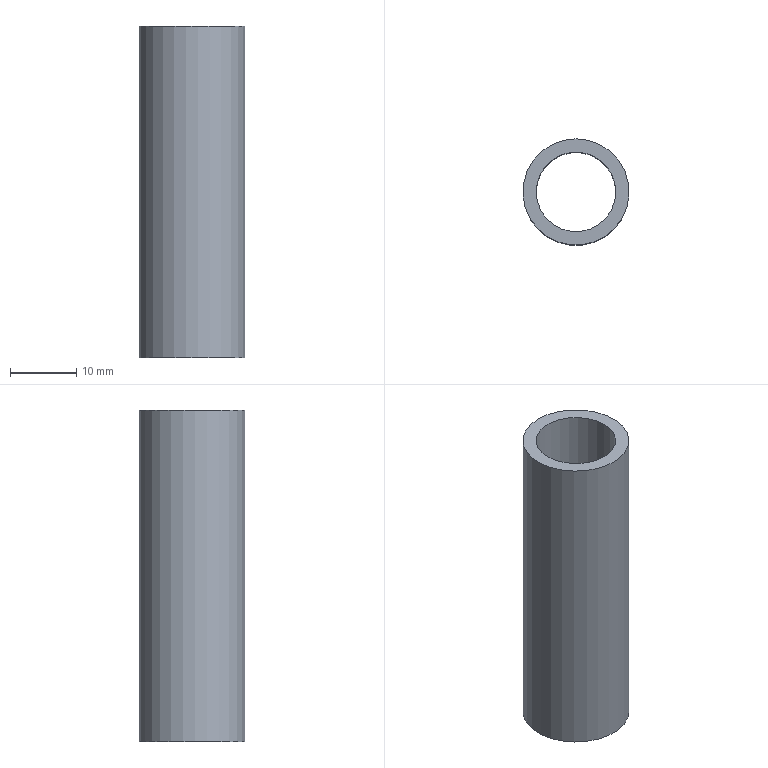Part | NX | features solid 2 | 1 solid | 4 faces | box 16 x 16 x 50 mm | volume 4398 mm3 | plane 2 | cylinder 2 | commonest cylinder face diameters 12 x1 16 x1
STEP:
#1=CARTESIAN_POINT('',(1206.,-380.,0.));
#2=VERTEX_POINT('',#1);
#3=CARTESIAN_POINT('',(1200.,-380.,0.));
#4=DIRECTION('',(0.,0.,1.));
#5=DIRECTION('',(1.,0.,0.));
#6=AXIS2_PLACEMENT_3D('',#3,#4,#5);
#7=CIRCLE('',#6,6.);
#8=EDGE_CURVE('',#2,#2,#7,.F.);
#9=ORIENTED_EDGE('',*,*,#8,.T.);
#10=EDGE_LOOP('',(#9));
#11=FACE_BOUND('',#10,.T.);
#12=CARTESIAN_POINT('',(1200.,-372.,0.));
#13=VERTEX_POINT('',#12);
#14=CARTESIAN_POINT('',(1200.,-380.,0.));
#15=DIRECTION('',(0.,0.,-1.));
#16=DIRECTION('',(0.,1.,0.));
#17=AXIS2_PLACEMENT_3D('',#14,#15,#16);
#18=CIRCLE('',#17,8.);
#19=EDGE_CURVE('',#13,#13,#18,.T.);
#20=ORIENTED_EDGE('',*,*,#19,.F.);
#21=EDGE_LOOP('',(#20));
#22=FACE_BOUND('',#21,.T.);
#23=CARTESIAN_POINT('',(1200.,-380.,0.));
#24=DIRECTION('',(0.,0.,1.));
#25=DIRECTION('',(0.,-1.,0.));
#26=AXIS2_PLACEMENT_3D('',#23,#24,#25);
#27=PLANE('',#26);
#28=ADVANCED_FACE('',(#11,#22),#27,.T.);
#29=CARTESIAN_POINT('',(1206.,-380.,-50.));
#30=VERTEX_POINT('',#29);
#31=CARTESIAN_POINT('',(1200.,-380.,-50.));
#32=DIRECTION('',(0.,0.,1.));
#33=DIRECTION('',(1.,0.,0.));
#34=AXIS2_PLACEMENT_3D('',#31,#32,#33);
#35=CIRCLE('',#34,6.);
#36=EDGE_CURVE('',#30,#30,#35,.F.);
#37=ORIENTED_EDGE('',*,*,#36,.F.);
#38=EDGE_LOOP('',(#37));
#39=FACE_BOUND('',#38,.T.);
#40=CARTESIAN_POINT('',(1200.,-372.,-50.));
#41=VERTEX_POINT('',#40);
#42=CARTESIAN_POINT('',(1200.,-380.,-50.));
#43=DIRECTION('',(0.,0.,-1.));
#44=DIRECTION('',(0.,1.,0.));
#45=AXIS2_PLACEMENT_3D('',#42,#43,#44);
#46=CIRCLE('',#45,8.);
#47=EDGE_CURVE('',#41,#41,#46,.T.);
#48=ORIENTED_EDGE('',*,*,#47,.T.);
#49=EDGE_LOOP('',(#48));
#50=FACE_BOUND('',#49,.T.);
#51=CARTESIAN_POINT('',(1200.,-380.,-50.));
#52=DIRECTION('',(0.,0.,1.));
#53=DIRECTION('',(0.,-1.,0.));
#54=AXIS2_PLACEMENT_3D('',#51,#52,#53);
#55=PLANE('',#54);
#56=ADVANCED_FACE('',(#39,#50),#55,.F.);
#57=ORIENTED_EDGE('',*,*,#8,.F.);
#58=EDGE_LOOP('',(#57));
#59=FACE_BOUND('',#58,.T.);
#60=ORIENTED_EDGE('',*,*,#36,.T.);
#61=EDGE_LOOP('',(#60));
#62=FACE_BOUND('',#61,.T.);
#63=CARTESIAN_POINT('',(1200.,-380.,-50.));
#64=DIRECTION('',(0.,0.,1.));
#65=DIRECTION('',(1.,0.,0.));
#66=AXIS2_PLACEMENT_3D('',#63,#64,#65);
#67=CYLINDRICAL_SURFACE('',#66,6.);
#68=ADVANCED_FACE('',(#59,#62),#67,.F.);
#69=ORIENTED_EDGE('',*,*,#19,.T.);
#70=EDGE_LOOP('',(#69));
#71=FACE_BOUND('',#70,.T.);
#72=ORIENTED_EDGE('',*,*,#47,.F.);
#73=EDGE_LOOP('',(#72));
#74=FACE_BOUND('',#73,.T.);
#75=CARTESIAN_POINT('',(1200.,-380.,-50.));
#76=DIRECTION('',(0.,0.,1.));
#77=DIRECTION('',(1.,0.,0.));
#78=AXIS2_PLACEMENT_3D('',#75,#76,#77);
#79=CYLINDRICAL_SURFACE('',#78,8.);
#80=ADVANCED_FACE('',(#71,#74),#79,.T.);
#81=CLOSED_SHELL('',(#28,#56,#68,#80));
#82=MANIFOLD_SOLID_BREP('',#81);
#83=(LENGTH_UNIT()NAMED_UNIT(*)SI_UNIT(.MILLI.,.METRE.));
#84=UNCERTAINTY_MEASURE_WITH_UNIT(LENGTH_MEASURE(0.00001),#83,'','');
#85=(NAMED_UNIT(*)PLANE_ANGLE_UNIT()SI_UNIT($,.RADIAN.));
#86=(NAMED_UNIT(*)SI_UNIT($,.STERADIAN.)SOLID_ANGLE_UNIT());
#87=(GEOMETRIC_REPRESENTATION_CONTEXT(3)GLOBAL_UNCERTAINTY_ASSIGNED_CONTEXT((#84))GLOBAL_UNIT_ASSIGNED_CONTEXT((#83,#85,#86))REPRESENTATION_CONTEXT('',''));
#88=ADVANCED_BREP_SHAPE_REPRESENTATION('',(#82),#87);